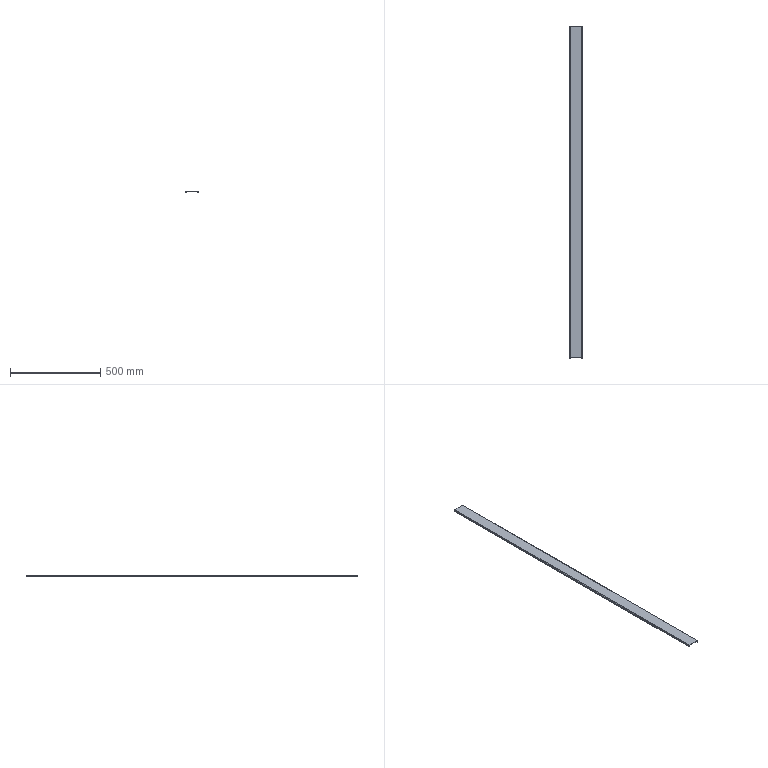Part | SolidWorks | features BaseBody 1 | 1 solid | 22 faces | box 67 x 1838 x 10 mm | volume 369847 mm3 | plane 18 | cylinder 4 | commonest cylinder face diameters 1 x2 6 x2
STEP:
#1=CARTESIAN_POINT('',(-31.,918.9,-10.));
#2=VERTEX_POINT('',#1);
#3=CARTESIAN_POINT('',(-31.,-918.9,-10.));
#4=VERTEX_POINT('',#3);
#5=CARTESIAN_POINT('',(-31.,-918.9,-10.));
#6=DIRECTION('',(0.,-1.,0.));
#7=VECTOR('',#6,1000.);
#8=LINE('',#5,#7);
#9=EDGE_CURVE('',#2,#4,#8,.T.);
#10=ORIENTED_EDGE('',*,*,#9,.T.);
#11=CARTESIAN_POINT('',(-33.5,-918.9,-10.));
#12=VERTEX_POINT('',#11);
#13=CARTESIAN_POINT('',(-33.5,-918.9,-10.));
#14=DIRECTION('',(1.,0.,0.));
#15=VECTOR('',#14,1000.);
#16=LINE('',#13,#15);
#17=EDGE_CURVE('',#12,#4,#16,.T.);
#18=ORIENTED_EDGE('',*,*,#17,.F.);
#19=CARTESIAN_POINT('',(-33.5,918.9,-10.));
#20=VERTEX_POINT('',#19);
#21=CARTESIAN_POINT('',(-33.5,0.,-10.));
#22=DIRECTION('',(0.,-1.,0.));
#23=VECTOR('',#22,1000.);
#24=LINE('',#21,#23);
#25=EDGE_CURVE('',#20,#12,#24,.T.);
#26=ORIENTED_EDGE('',*,*,#25,.F.);
#27=CARTESIAN_POINT('',(-33.5,918.9,-10.));
#28=DIRECTION('',(1.,0.,0.));
#29=VECTOR('',#28,1000.);
#30=LINE('',#27,#29);
#31=EDGE_CURVE('',#20,#2,#30,.T.);
#32=ORIENTED_EDGE('',*,*,#31,.T.);
#33=EDGE_LOOP('',(#10,#18,#26,#32));
#34=FACE_OUTER_BOUND('',#33,.T.);
#35=CARTESIAN_POINT('',(-33.5,-918.9,-10.));
#36=DIRECTION('',(0.,0.,1.));
#37=DIRECTION('',(1.,0.,0.));
#38=AXIS2_PLACEMENT_3D('',#35,#36,#37);
#39=PLANE('',#38);
#40=ADVANCED_FACE('',(#34),#39,.F.);
#41=CARTESIAN_POINT('',(-31.,918.9,-3.));
#42=VERTEX_POINT('',#41);
#43=CARTESIAN_POINT('',(-31.,918.9,-10.));
#44=DIRECTION('',(0.,0.,-1.));
#45=VECTOR('',#44,1000.);
#46=LINE('',#43,#45);
#47=EDGE_CURVE('',#42,#2,#46,.T.);
#48=ORIENTED_EDGE('',*,*,#47,.F.);
#49=CARTESIAN_POINT('',(-31.,-918.9,-3.));
#50=VERTEX_POINT('',#49);
#51=CARTESIAN_POINT('',(-31.,-918.9,-3.));
#52=DIRECTION('',(0.,1.,0.));
#53=VECTOR('',#52,1000.);
#54=LINE('',#51,#53);
#55=EDGE_CURVE('',#50,#42,#54,.T.);
#56=ORIENTED_EDGE('',*,*,#55,.F.);
#57=CARTESIAN_POINT('',(-31.,-918.9,-2.5));
#58=DIRECTION('',(0.,0.,1.));
#59=VECTOR('',#58,1000.);
#60=LINE('',#57,#59);
#61=EDGE_CURVE('',#4,#50,#60,.T.);
#62=ORIENTED_EDGE('',*,*,#61,.F.);
#63=ORIENTED_EDGE('',*,*,#9,.F.);
#64=EDGE_LOOP('',(#48,#56,#62,#63));
#65=FACE_OUTER_BOUND('',#64,.T.);
#66=CARTESIAN_POINT('',(-31.,0.,0.));
#67=DIRECTION('',(1.,0.,0.));
#68=DIRECTION('',(0.,0.,-1.));
#69=AXIS2_PLACEMENT_3D('',#66,#67,#68);
#70=PLANE('',#69);
#71=ADVANCED_FACE('',(#65),#70,.T.);
#72=CARTESIAN_POINT('',(-33.5,918.9,-3.));
#73=VERTEX_POINT('',#72);
#74=CARTESIAN_POINT('',(-33.5,-918.9,-3.));
#75=VERTEX_POINT('',#74);
#76=CARTESIAN_POINT('',(-33.5,-918.9,-3.));
#77=DIRECTION('',(0.,-1.,0.));
#78=VECTOR('',#77,1000.);
#79=LINE('',#76,#78);
#80=EDGE_CURVE('',#73,#75,#79,.T.);
#81=ORIENTED_EDGE('',*,*,#80,.F.);
#82=CARTESIAN_POINT('',(-33.5,918.9,0.));
#83=DIRECTION('',(0.,0.,-1.));
#84=VECTOR('',#83,1000.);
#85=LINE('',#82,#84);
#86=EDGE_CURVE('',#73,#20,#85,.T.);
#87=ORIENTED_EDGE('',*,*,#86,.T.);
#88=ORIENTED_EDGE('',*,*,#25,.T.);
#89=CARTESIAN_POINT('',(-33.5,-918.9,0.));
#90=DIRECTION('',(0.,0.,1.));
#91=VECTOR('',#90,1000.);
#92=LINE('',#89,#91);
#93=EDGE_CURVE('',#12,#75,#92,.T.);
#94=ORIENTED_EDGE('',*,*,#93,.T.);
#95=EDGE_LOOP('',(#81,#87,#88,#94));
#96=FACE_OUTER_BOUND('',#95,.T.);
#97=CARTESIAN_POINT('',(-33.5,0.,0.));
#98=DIRECTION('',(1.,0.,0.));
#99=DIRECTION('',(0.,0.,-1.));
#100=AXIS2_PLACEMENT_3D('',#97,#98,#99);
#101=PLANE('',#100);
#102=ADVANCED_FACE('',(#96),#101,.F.);
#103=CARTESIAN_POINT('',(-33.5,-918.9,-3.));
#104=DIRECTION('',(-1.,0.,0.));
#105=VECTOR('',#104,1000.);
#106=LINE('',#103,#105);
#107=EDGE_CURVE('',#50,#75,#106,.T.);
#108=ORIENTED_EDGE('',*,*,#107,.T.);
#109=ORIENTED_EDGE('',*,*,#93,.F.);
#110=ORIENTED_EDGE('',*,*,#17,.T.);
#111=ORIENTED_EDGE('',*,*,#61,.T.);
#112=EDGE_LOOP('',(#108,#109,#110,#111));
#113=FACE_OUTER_BOUND('',#112,.T.);
#114=CARTESIAN_POINT('',(-33.5,-918.9,-2.5));
#115=DIRECTION('',(0.,1.,0.));
#116=DIRECTION('',(1.,0.,0.));
#117=AXIS2_PLACEMENT_3D('',#114,#115,#116);
#118=PLANE('',#117);
#119=ADVANCED_FACE('',(#113),#118,.F.);
#120=CARTESIAN_POINT('',(-31.,918.9,-3.));
#121=DIRECTION('',(-1.,0.,0.));
#122=VECTOR('',#121,1000.);
#123=LINE('',#120,#122);
#124=EDGE_CURVE('',#42,#73,#123,.T.);
#125=ORIENTED_EDGE('',*,*,#124,.F.);
#126=ORIENTED_EDGE('',*,*,#47,.T.);
#127=ORIENTED_EDGE('',*,*,#31,.F.);
#128=ORIENTED_EDGE('',*,*,#86,.F.);
#129=EDGE_LOOP('',(#125,#126,#127,#128));
#130=FACE_OUTER_BOUND('',#129,.T.);
#131=CARTESIAN_POINT('',(-33.5,918.9,-10.));
#132=DIRECTION('',(0.,-1.,0.));
#133=DIRECTION('',(0.,0.,-1.));
#134=AXIS2_PLACEMENT_3D('',#131,#132,#133);
#135=PLANE('',#134);
#136=ADVANCED_FACE('',(#130),#135,.F.);
#137=CARTESIAN_POINT('',(-30.5,918.9,-2.5));
#138=VERTEX_POINT('',#137);
#139=CARTESIAN_POINT('',(-30.5,-918.9,-2.5));
#140=VERTEX_POINT('',#139);
#141=CARTESIAN_POINT('',(-30.5,918.9,-2.5));
#142=DIRECTION('',(0.,-1.,0.));
#143=VECTOR('',#142,1000.);
#144=LINE('',#141,#143);
#145=EDGE_CURVE('',#138,#140,#144,.T.);
#146=ORIENTED_EDGE('',*,*,#145,.T.);
#147=CARTESIAN_POINT('',(-30.5,-918.9,-3.));
#148=DIRECTION('',(0.,-1.,0.));
#149=DIRECTION('',(0.,0.,1.));
#150=AXIS2_PLACEMENT_3D('',#147,#148,#149);
#151=CIRCLE('',#150,0.5);
#152=EDGE_CURVE('',#140,#50,#151,.T.);
#153=ORIENTED_EDGE('',*,*,#152,.T.);
#154=ORIENTED_EDGE('',*,*,#55,.T.);
#155=CARTESIAN_POINT('',(-30.5,918.9,-3.));
#156=DIRECTION('',(0.,1.,0.));
#157=DIRECTION('',(0.,0.,1.));
#158=AXIS2_PLACEMENT_3D('',#155,#156,#157);
#159=CIRCLE('',#158,0.5);
#160=EDGE_CURVE('',#42,#138,#159,.T.);
#161=ORIENTED_EDGE('',*,*,#160,.T.);
#162=EDGE_LOOP('',(#146,#153,#154,#161));
#163=FACE_OUTER_BOUND('',#162,.T.);
#164=CARTESIAN_POINT('',(-30.5,918.9,-3.));
#165=DIRECTION('',(0.,1.,0.));
#166=DIRECTION('',(-1.,0.,0.));
#167=AXIS2_PLACEMENT_3D('',#164,#165,#166);
#168=CYLINDRICAL_SURFACE('',#167,0.5);
#169=ADVANCED_FACE('',(#163),#168,.F.);
#170=CARTESIAN_POINT('',(-30.5,918.9,0.));
#171=VERTEX_POINT('',#170);
#172=CARTESIAN_POINT('',(-30.5,-918.9,0.));
#173=VERTEX_POINT('',#172);
#174=CARTESIAN_POINT('',(-30.5,918.9,0.));
#175=DIRECTION('',(0.,-1.,0.));
#176=VECTOR('',#175,1000.);
#177=LINE('',#174,#176);
#178=EDGE_CURVE('',#171,#173,#177,.T.);
#179=ORIENTED_EDGE('',*,*,#178,.F.);
#180=CARTESIAN_POINT('',(-30.5,918.9,-3.));
#181=DIRECTION('',(0.,1.,0.));
#182=DIRECTION('',(0.,0.,1.));
#183=AXIS2_PLACEMENT_3D('',#180,#181,#182);
#184=CIRCLE('',#183,3.);
#185=EDGE_CURVE('',#73,#171,#184,.T.);
#186=ORIENTED_EDGE('',*,*,#185,.F.);
#187=ORIENTED_EDGE('',*,*,#80,.T.);
#188=CARTESIAN_POINT('',(-30.5,-918.9,-3.));
#189=DIRECTION('',(0.,-1.,0.));
#190=DIRECTION('',(0.,0.,1.));
#191=AXIS2_PLACEMENT_3D('',#188,#189,#190);
#192=CIRCLE('',#191,3.);
#193=EDGE_CURVE('',#173,#75,#192,.T.);
#194=ORIENTED_EDGE('',*,*,#193,.F.);
#195=EDGE_LOOP('',(#179,#186,#187,#194));
#196=FACE_OUTER_BOUND('',#195,.T.);
#197=CARTESIAN_POINT('',(-30.5,918.9,-3.));
#198=DIRECTION('',(0.,1.,0.));
#199=DIRECTION('',(-1.,0.,0.));
#200=AXIS2_PLACEMENT_3D('',#197,#198,#199);
#201=CYLINDRICAL_SURFACE('',#200,3.);
#202=ADVANCED_FACE('',(#196),#201,.T.);
#203=ORIENTED_EDGE('',*,*,#160,.F.);
#204=ORIENTED_EDGE('',*,*,#124,.T.);
#205=ORIENTED_EDGE('',*,*,#185,.T.);
#206=CARTESIAN_POINT('',(-30.5,918.9,-2.5));
#207=DIRECTION('',(0.,0.,1.));
#208=VECTOR('',#207,1000.);
#209=LINE('',#206,#208);
#210=EDGE_CURVE('',#138,#171,#209,.T.);
#211=ORIENTED_EDGE('',*,*,#210,.F.);
#212=EDGE_LOOP('',(#203,#204,#205,#211));
#213=FACE_OUTER_BOUND('',#212,.T.);
#214=CARTESIAN_POINT('',(-30.5,918.9,-3.));
#215=DIRECTION('',(0.,-1.,0.));
#216=DIRECTION('',(0.,0.,-1.));
#217=AXIS2_PLACEMENT_3D('',#214,#215,#216);
#218=PLANE('',#217);
#219=ADVANCED_FACE('',(#213),#218,.F.);
#220=ORIENTED_EDGE('',*,*,#107,.F.);
#221=ORIENTED_EDGE('',*,*,#152,.F.);
#222=CARTESIAN_POINT('',(-30.5,-918.9,-2.5));
#223=DIRECTION('',(0.,0.,1.));
#224=VECTOR('',#223,1000.);
#225=LINE('',#222,#224);
#226=EDGE_CURVE('',#140,#173,#225,.T.);
#227=ORIENTED_EDGE('',*,*,#226,.T.);
#228=ORIENTED_EDGE('',*,*,#193,.T.);
#229=EDGE_LOOP('',(#220,#221,#227,#228));
#230=FACE_OUTER_BOUND('',#229,.T.);
#231=CARTESIAN_POINT('',(-30.5,-918.9,-3.));
#232=DIRECTION('',(0.,-1.,0.));
#233=DIRECTION('',(0.,0.,-1.));
#234=AXIS2_PLACEMENT_3D('',#231,#232,#233);
#235=PLANE('',#234);
#236=ADVANCED_FACE('',(#230),#235,.T.);
#237=CARTESIAN_POINT('',(31.,-918.9,-10.));
#238=VERTEX_POINT('',#237);
#239=CARTESIAN_POINT('',(31.,918.9,-10.));
#240=VERTEX_POINT('',#239);
#241=CARTESIAN_POINT('',(31.,918.9,-10.));
#242=DIRECTION('',(0.,1.,0.));
#243=VECTOR('',#242,1000.);
#244=LINE('',#241,#243);
#245=EDGE_CURVE('',#238,#240,#244,.T.);
#246=ORIENTED_EDGE('',*,*,#245,.T.);
#247=CARTESIAN_POINT('',(33.5,918.9,-10.));
#248=VERTEX_POINT('',#247);
#249=CARTESIAN_POINT('',(33.5,918.9,-10.));
#250=DIRECTION('',(-1.,0.,0.));
#251=VECTOR('',#250,1000.);
#252=LINE('',#249,#251);
#253=EDGE_CURVE('',#248,#240,#252,.T.);
#254=ORIENTED_EDGE('',*,*,#253,.F.);
#255=CARTESIAN_POINT('',(33.5,-918.9,-10.));
#256=VERTEX_POINT('',#255);
#257=CARTESIAN_POINT('',(33.5,0.,-10.));
#258=DIRECTION('',(0.,1.,0.));
#259=VECTOR('',#258,1000.);
#260=LINE('',#257,#259);
#261=EDGE_CURVE('',#256,#248,#260,.T.);
#262=ORIENTED_EDGE('',*,*,#261,.F.);
#263=CARTESIAN_POINT('',(33.5,-918.9,-10.));
#264=DIRECTION('',(-1.,0.,0.));
#265=VECTOR('',#264,1000.);
#266=LINE('',#263,#265);
#267=EDGE_CURVE('',#256,#238,#266,.T.);
#268=ORIENTED_EDGE('',*,*,#267,.T.);
#269=EDGE_LOOP('',(#246,#254,#262,#268));
#270=FACE_OUTER_BOUND('',#269,.T.);
#271=CARTESIAN_POINT('',(33.5,918.9,-10.));
#272=DIRECTION('',(0.,0.,1.));
#273=DIRECTION('',(1.,0.,0.));
#274=AXIS2_PLACEMENT_3D('',#271,#272,#273);
#275=PLANE('',#274);
#276=ADVANCED_FACE('',(#270),#275,.F.);
#277=CARTESIAN_POINT('',(31.,-918.9,-3.));
#278=VERTEX_POINT('',#277);
#279=CARTESIAN_POINT('',(31.,-918.9,-10.));
#280=DIRECTION('',(0.,0.,-1.));
#281=VECTOR('',#280,1000.);
#282=LINE('',#279,#281);
#283=EDGE_CURVE('',#278,#238,#282,.T.);
#284=ORIENTED_EDGE('',*,*,#283,.F.);
#285=CARTESIAN_POINT('',(31.,918.9,-3.));
#286=VERTEX_POINT('',#285);
#287=CARTESIAN_POINT('',(31.,918.9,-3.));
#288=DIRECTION('',(0.,-1.,0.));
#289=VECTOR('',#288,1000.);
#290=LINE('',#287,#289);
#291=EDGE_CURVE('',#286,#278,#290,.T.);
#292=ORIENTED_EDGE('',*,*,#291,.F.);
#293=CARTESIAN_POINT('',(31.,918.9,-2.5));
#294=DIRECTION('',(0.,0.,1.));
#295=VECTOR('',#294,1000.);
#296=LINE('',#293,#295);
#297=EDGE_CURVE('',#240,#286,#296,.T.);
#298=ORIENTED_EDGE('',*,*,#297,.F.);
#299=ORIENTED_EDGE('',*,*,#245,.F.);
#300=EDGE_LOOP('',(#284,#292,#298,#299));
#301=FACE_OUTER_BOUND('',#300,.T.);
#302=CARTESIAN_POINT('',(31.,0.,0.));
#303=DIRECTION('',(-1.,0.,0.));
#304=DIRECTION('',(0.,0.,1.));
#305=AXIS2_PLACEMENT_3D('',#302,#303,#304);
#306=PLANE('',#305);
#307=ADVANCED_FACE('',(#301),#306,.T.);
#308=CARTESIAN_POINT('',(33.5,-918.9,-3.));
#309=VERTEX_POINT('',#308);
#310=CARTESIAN_POINT('',(33.5,918.9,-3.));
#311=VERTEX_POINT('',#310);
#312=CARTESIAN_POINT('',(33.5,918.9,-3.));
#313=DIRECTION('',(0.,1.,0.));
#314=VECTOR('',#313,1000.);
#315=LINE('',#312,#314);
#316=EDGE_CURVE('',#309,#311,#315,.T.);
#317=ORIENTED_EDGE('',*,*,#316,.F.);
#318=CARTESIAN_POINT('',(33.5,-918.9,0.));
#319=DIRECTION('',(0.,0.,-1.));
#320=VECTOR('',#319,1000.);
#321=LINE('',#318,#320);
#322=EDGE_CURVE('',#309,#256,#321,.T.);
#323=ORIENTED_EDGE('',*,*,#322,.T.);
#324=ORIENTED_EDGE('',*,*,#261,.T.);
#325=CARTESIAN_POINT('',(33.5,918.9,0.));
#326=DIRECTION('',(0.,0.,1.));
#327=VECTOR('',#326,1000.);
#328=LINE('',#325,#327);
#329=EDGE_CURVE('',#248,#311,#328,.T.);
#330=ORIENTED_EDGE('',*,*,#329,.T.);
#331=EDGE_LOOP('',(#317,#323,#324,#330));
#332=FACE_OUTER_BOUND('',#331,.T.);
#333=CARTESIAN_POINT('',(33.5,0.,0.));
#334=DIRECTION('',(-1.,0.,0.));
#335=DIRECTION('',(0.,0.,1.));
#336=AXIS2_PLACEMENT_3D('',#333,#334,#335);
#337=PLANE('',#336);
#338=ADVANCED_FACE('',(#332),#337,.F.);
#339=CARTESIAN_POINT('',(33.5,918.9,-3.));
#340=DIRECTION('',(1.,0.,0.));
#341=VECTOR('',#340,1000.);
#342=LINE('',#339,#341);
#343=EDGE_CURVE('',#286,#311,#342,.T.);
#344=ORIENTED_EDGE('',*,*,#343,.T.);
#345=ORIENTED_EDGE('',*,*,#329,.F.);
#346=ORIENTED_EDGE('',*,*,#253,.T.);
#347=ORIENTED_EDGE('',*,*,#297,.T.);
#348=EDGE_LOOP('',(#344,#345,#346,#347));
#349=FACE_OUTER_BOUND('',#348,.T.);
#350=CARTESIAN_POINT('',(33.5,918.9,-2.5));
#351=DIRECTION('',(0.,-1.,0.));
#352=DIRECTION('',(0.,0.,-1.));
#353=AXIS2_PLACEMENT_3D('',#350,#351,#352);
#354=PLANE('',#353);
#355=ADVANCED_FACE('',(#349),#354,.F.);
#356=CARTESIAN_POINT('',(31.,-918.9,-3.));
#357=DIRECTION('',(1.,0.,0.));
#358=VECTOR('',#357,1000.);
#359=LINE('',#356,#358);
#360=EDGE_CURVE('',#278,#309,#359,.T.);
#361=ORIENTED_EDGE('',*,*,#360,.F.);
#362=ORIENTED_EDGE('',*,*,#283,.T.);
#363=ORIENTED_EDGE('',*,*,#267,.F.);
#364=ORIENTED_EDGE('',*,*,#322,.F.);
#365=EDGE_LOOP('',(#361,#362,#363,#364));
#366=FACE_OUTER_BOUND('',#365,.T.);
#367=CARTESIAN_POINT('',(33.5,-918.9,-10.));
#368=DIRECTION('',(0.,1.,0.));
#369=DIRECTION('',(1.,0.,0.));
#370=AXIS2_PLACEMENT_3D('',#367,#368,#369);
#371=PLANE('',#370);
#372=ADVANCED_FACE('',(#366),#371,.F.);
#373=CARTESIAN_POINT('',(30.5,-918.9,-2.5));
#374=VERTEX_POINT('',#373);
#375=CARTESIAN_POINT('',(30.5,918.9,-2.5));
#376=VERTEX_POINT('',#375);
#377=CARTESIAN_POINT('',(30.5,-918.9,-2.5));
#378=DIRECTION('',(0.,1.,0.));
#379=VECTOR('',#378,1000.);
#380=LINE('',#377,#379);
#381=EDGE_CURVE('',#374,#376,#380,.T.);
#382=ORIENTED_EDGE('',*,*,#381,.T.);
#383=CARTESIAN_POINT('',(30.5,918.9,-3.));
#384=DIRECTION('',(0.,1.,0.));
#385=DIRECTION('',(0.,0.,-1.));
#386=AXIS2_PLACEMENT_3D('',#383,#384,#385);
#387=CIRCLE('',#386,0.5);
#388=EDGE_CURVE('',#376,#286,#387,.T.);
#389=ORIENTED_EDGE('',*,*,#388,.T.);
#390=ORIENTED_EDGE('',*,*,#291,.T.);
#391=CARTESIAN_POINT('',(30.5,-918.9,-3.));
#392=DIRECTION('',(0.,-1.,0.));
#393=DIRECTION('',(0.,0.,-1.));
#394=AXIS2_PLACEMENT_3D('',#391,#392,#393);
#395=CIRCLE('',#394,0.5);
#396=EDGE_CURVE('',#278,#374,#395,.T.);
#397=ORIENTED_EDGE('',*,*,#396,.T.);
#398=EDGE_LOOP('',(#382,#389,#390,#397));
#399=FACE_OUTER_BOUND('',#398,.T.);
#400=CARTESIAN_POINT('',(30.5,-918.9,-3.));
#401=DIRECTION('',(0.,-1.,0.));
#402=DIRECTION('',(1.,0.,0.));
#403=AXIS2_PLACEMENT_3D('',#400,#401,#402);
#404=CYLINDRICAL_SURFACE('',#403,0.5);
#405=ADVANCED_FACE('',(#399),#404,.F.);
#406=CARTESIAN_POINT('',(30.5,-918.9,0.));
#407=VERTEX_POINT('',#406);
#408=CARTESIAN_POINT('',(30.5,918.9,0.));
#409=VERTEX_POINT('',#408);
#410=CARTESIAN_POINT('',(30.5,-918.9,0.));
#411=DIRECTION('',(0.,1.,0.));
#412=VECTOR('',#411,1000.);
#413=LINE('',#410,#412);
#414=EDGE_CURVE('',#407,#409,#413,.T.);
#415=ORIENTED_EDGE('',*,*,#414,.F.);
#416=CARTESIAN_POINT('',(30.5,-918.9,-3.));
#417=DIRECTION('',(0.,-1.,0.));
#418=DIRECTION('',(0.,0.,-1.));
#419=AXIS2_PLACEMENT_3D('',#416,#417,#418);
#420=CIRCLE('',#419,3.);
#421=EDGE_CURVE('',#309,#407,#420,.T.);
#422=ORIENTED_EDGE('',*,*,#421,.F.);
#423=ORIENTED_EDGE('',*,*,#316,.T.);
#424=CARTESIAN_POINT('',(30.5,918.9,-3.));
#425=DIRECTION('',(0.,1.,0.));
#426=DIRECTION('',(0.,0.,-1.));
#427=AXIS2_PLACEMENT_3D('',#424,#425,#426);
#428=CIRCLE('',#427,3.);
#429=EDGE_CURVE('',#409,#311,#428,.T.);
#430=ORIENTED_EDGE('',*,*,#429,.F.);
#431=EDGE_LOOP('',(#415,#422,#423,#430));
#432=FACE_OUTER_BOUND('',#431,.T.);
#433=CARTESIAN_POINT('',(30.5,-918.9,-3.));
#434=DIRECTION('',(0.,-1.,0.));
#435=DIRECTION('',(1.,0.,0.));
#436=AXIS2_PLACEMENT_3D('',#433,#434,#435);
#437=CYLINDRICAL_SURFACE('',#436,3.);
#438=ADVANCED_FACE('',(#432),#437,.T.);
#439=ORIENTED_EDGE('',*,*,#396,.F.);
#440=ORIENTED_EDGE('',*,*,#360,.T.);
#441=ORIENTED_EDGE('',*,*,#421,.T.);
#442=CARTESIAN_POINT('',(30.5,-918.9,-2.5));
#443=DIRECTION('',(0.,0.,1.));
#444=VECTOR('',#443,1000.);
#445=LINE('',#442,#444);
#446=EDGE_CURVE('',#374,#407,#445,.T.);
#447=ORIENTED_EDGE('',*,*,#446,.F.);
#448=EDGE_LOOP('',(#439,#440,#441,#447));
#449=FACE_OUTER_BOUND('',#448,.T.);
#450=CARTESIAN_POINT('',(30.5,-918.9,-3.));
#451=DIRECTION('',(0.,1.,0.));
#452=DIRECTION('',(1.,0.,0.));
#453=AXIS2_PLACEMENT_3D('',#450,#451,#452);
#454=PLANE('',#453);
#455=ADVANCED_FACE('',(#449),#454,.F.);
#456=ORIENTED_EDGE('',*,*,#343,.F.);
#457=ORIENTED_EDGE('',*,*,#388,.F.);
#458=CARTESIAN_POINT('',(30.5,918.9,-2.5));
#459=DIRECTION('',(0.,0.,1.));
#460=VECTOR('',#459,1000.);
#461=LINE('',#458,#460);
#462=EDGE_CURVE('',#376,#409,#461,.T.);
#463=ORIENTED_EDGE('',*,*,#462,.T.);
#464=ORIENTED_EDGE('',*,*,#429,.T.);
#465=EDGE_LOOP('',(#456,#457,#463,#464));
#466=FACE_OUTER_BOUND('',#465,.T.);
#467=CARTESIAN_POINT('',(30.5,918.9,-3.));
#468=DIRECTION('',(0.,1.,0.));
#469=DIRECTION('',(1.,0.,0.));
#470=AXIS2_PLACEMENT_3D('',#467,#468,#469);
#471=PLANE('',#470);
#472=ADVANCED_FACE('',(#466),#471,.T.);
#473=ORIENTED_EDGE('',*,*,#226,.F.);
#474=CARTESIAN_POINT('',(33.5,-918.9,-2.5));
#475=DIRECTION('',(1.,0.,0.));
#476=VECTOR('',#475,1000.);
#477=LINE('',#474,#476);
#478=EDGE_CURVE('',#140,#374,#477,.T.);
#479=ORIENTED_EDGE('',*,*,#478,.T.);
#480=ORIENTED_EDGE('',*,*,#446,.T.);
#481=CARTESIAN_POINT('',(33.5,-918.9,0.));
#482=DIRECTION('',(1.,0.,0.));
#483=VECTOR('',#482,1000.);
#484=LINE('',#481,#483);
#485=EDGE_CURVE('',#173,#407,#484,.T.);
#486=ORIENTED_EDGE('',*,*,#485,.F.);
#487=EDGE_LOOP('',(#473,#479,#480,#486));
#488=FACE_OUTER_BOUND('',#487,.T.);
#489=CARTESIAN_POINT('',(33.5,-918.9,-2.5));
#490=DIRECTION('',(0.,-1.,0.));
#491=DIRECTION('',(0.,0.,-1.));
#492=AXIS2_PLACEMENT_3D('',#489,#490,#491);
#493=PLANE('',#492);
#494=ADVANCED_FACE('',(#488),#493,.T.);
#495=CARTESIAN_POINT('',(33.5,918.9,-2.5));
#496=DIRECTION('',(-1.,0.,0.));
#497=VECTOR('',#496,1000.);
#498=LINE('',#495,#497);
#499=EDGE_CURVE('',#376,#138,#498,.T.);
#500=ORIENTED_EDGE('',*,*,#499,.T.);
#501=ORIENTED_EDGE('',*,*,#210,.T.);
#502=CARTESIAN_POINT('',(33.5,918.9,0.));
#503=DIRECTION('',(-1.,0.,0.));
#504=VECTOR('',#503,1000.);
#505=LINE('',#502,#504);
#506=EDGE_CURVE('',#409,#171,#505,.T.);
#507=ORIENTED_EDGE('',*,*,#506,.F.);
#508=ORIENTED_EDGE('',*,*,#462,.F.);
#509=EDGE_LOOP('',(#500,#501,#507,#508));
#510=FACE_OUTER_BOUND('',#509,.T.);
#511=CARTESIAN_POINT('',(33.5,918.9,-2.5));
#512=DIRECTION('',(0.,1.,0.));
#513=DIRECTION('',(1.,0.,0.));
#514=AXIS2_PLACEMENT_3D('',#511,#512,#513);
#515=PLANE('',#514);
#516=ADVANCED_FACE('',(#510),#515,.T.);
#517=ORIENTED_EDGE('',*,*,#178,.T.);
#518=ORIENTED_EDGE('',*,*,#485,.T.);
#519=ORIENTED_EDGE('',*,*,#414,.T.);
#520=ORIENTED_EDGE('',*,*,#506,.T.);
#521=EDGE_LOOP('',(#517,#518,#519,#520));
#522=FACE_OUTER_BOUND('',#521,.T.);
#523=CARTESIAN_POINT('',(0.,0.,0.));
#524=DIRECTION('',(0.,0.,-1.));
#525=DIRECTION('',(0.,-1.,0.));
#526=AXIS2_PLACEMENT_3D('',#523,#524,#525);
#527=PLANE('',#526);
#528=ADVANCED_FACE('',(#522),#527,.F.);
#529=ORIENTED_EDGE('',*,*,#478,.F.);
#530=ORIENTED_EDGE('',*,*,#145,.F.);
#531=ORIENTED_EDGE('',*,*,#499,.F.);
#532=ORIENTED_EDGE('',*,*,#381,.F.);
#533=EDGE_LOOP('',(#529,#530,#531,#532));
#534=FACE_OUTER_BOUND('',#533,.T.);
#535=CARTESIAN_POINT('',(0.,0.,-2.5));
#536=DIRECTION('',(0.,0.,-1.));
#537=DIRECTION('',(0.,-1.,0.));
#538=AXIS2_PLACEMENT_3D('',#535,#536,#537);
#539=PLANE('',#538);
#540=ADVANCED_FACE('',(#534),#539,.T.);
#541=CLOSED_SHELL('',(#40,#71,#102,#119,#136,#169,#202,#219,#236,#276,#307,#338,#355,#372,#405,#438,#455,#472,#494,#516,#528,#540));
#542=MANIFOLD_SOLID_BREP('',#541);
#543=CARTESIAN_POINT('',(0.,0.,0.));
#544=DIRECTION('',(0.,0.,1.));
#545=DIRECTION('',(1.,0.,0.));
#546=AXIS2_PLACEMENT_3D('',#543,#544,#545);
#547=(LENGTH_UNIT()NAMED_UNIT(*)SI_UNIT(.MILLI.,.METRE.));
#548=UNCERTAINTY_MEASURE_WITH_UNIT(LENGTH_MEASURE(0.00001),#547,'','');
#549=(NAMED_UNIT(*)PLANE_ANGLE_UNIT()SI_UNIT($,.RADIAN.));
#550=(NAMED_UNIT(*)SI_UNIT($,.STERADIAN.)SOLID_ANGLE_UNIT());
#551=(GEOMETRIC_REPRESENTATION_CONTEXT(3)GLOBAL_UNCERTAINTY_ASSIGNED_CONTEXT((#548))GLOBAL_UNIT_ASSIGNED_CONTEXT((#547,#549,#550))REPRESENTATION_CONTEXT('',''));
#552=ADVANCED_BREP_SHAPE_REPRESENTATION('',(#542,#546),#551);